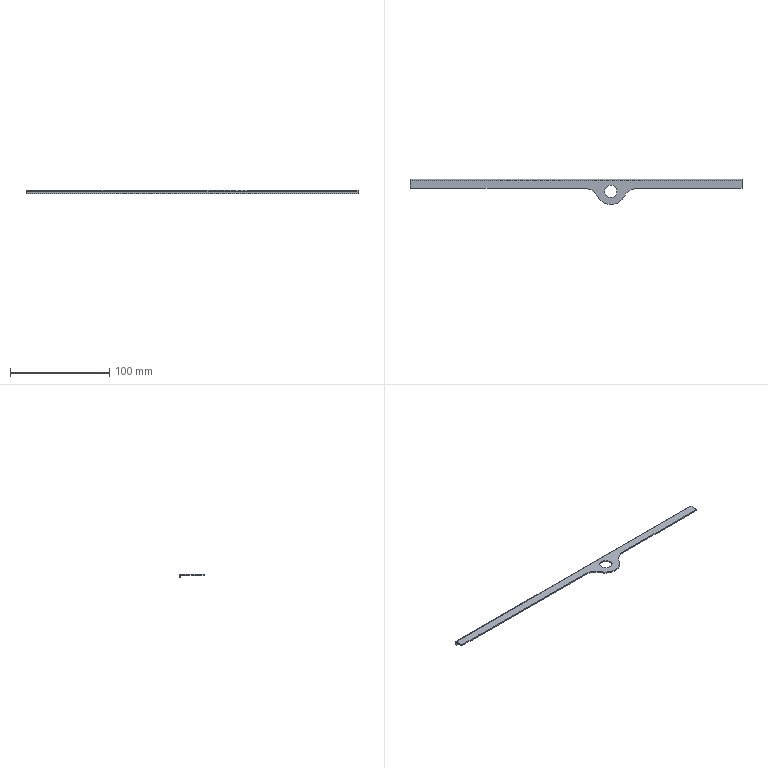Part | STEP file | gslz 2016.10.28-13_id1030_x_t | 1 solid | 17 faces | box 335 x 25.5 x 4 mm | volume 5252 mm3 | plane 10 | cylinder 7 | commonest cylinder face diameters 30 x3 4 x2 2 x1 12.3 x1
STEP:
#1=CARTESIAN_POINT('',(0.,0.,0.));
#2=DIRECTION('',(0.,0.,1.));
#3=DIRECTION('',(1.,0.,0.));
#4=AXIS2_PLACEMENT_3D('',#1,#2,#3);
#5=CARTESIAN_POINT('',(894.837,257.,0.));
#6=VERTEX_POINT('',#5);
#7=CARTESIAN_POINT('',(744.985,257.,0.));
#8=VERTEX_POINT('',#7);
#9=CARTESIAN_POINT('',(893.343,257.,0.));
#10=DIRECTION('',(-1.,0.,0.));
#11=VECTOR('',#10,1.);
#12=LINE('',#9,#11);
#13=CARTESIAN_POINT('',(893.343,257.,2.5));
#14=DIRECTION('',(0.,-1.,0.));
#15=DIRECTION('',(1.,0.,0.));
#16=AXIS2_PLACEMENT_3D('',#13,#14,#15);
#17=PLANE('',#16);
#18=CARTESIAN_POINT('',(0.,-2.5));
#19=DIRECTION('',(-1.,0.));
#20=VECTOR('',#19,1.);
#21=LINE('',#18,#20);
#22=(GEOMETRIC_REPRESENTATION_CONTEXT(2)PARAMETRIC_REPRESENTATION_CONTEXT()REPRESENTATION_CONTEXT('',''));
#23=DEFINITIONAL_REPRESENTATION('',(#21),#22);
#24=PCURVE('',#17,#23);
#25=CARTESIAN_POINT('',(3133.591,331.067,0.));
#26=DIRECTION('',(0.,0.,1.));
#27=DIRECTION('',(1.,0.,0.));
#28=AXIS2_PLACEMENT_3D('',#25,#26,#27);
#29=PLANE('',#28);
#30=CARTESIAN_POINT('',(-2240.248,-74.067));
#31=DIRECTION('',(-1.,0.));
#32=VECTOR('',#31,1.);
#33=LINE('',#30,#32);
#34=(GEOMETRIC_REPRESENTATION_CONTEXT(2)PARAMETRIC_REPRESENTATION_CONTEXT()REPRESENTATION_CONTEXT('',''));
#35=DEFINITIONAL_REPRESENTATION('',(#33),#34);
#36=PCURVE('',#29,#35);
#37=SURFACE_CURVE('',#12,(#24,#36),.PCURVE_S1.);
#38=EDGE_CURVE('',#6,#8,#37,.T.);
#39=ORIENTED_EDGE('',*,*,#38,.F.);
#40=CARTESIAN_POINT('',(894.837,257.,1.25));
#41=VERTEX_POINT('',#40);
#42=CARTESIAN_POINT('',(894.837,257.,2.5));
#43=DIRECTION('',(0.,0.,1.));
#44=VECTOR('',#43,1.);
#45=LINE('',#42,#44);
#46=CARTESIAN_POINT('',(1.493,0.));
#47=DIRECTION('',(0.,1.));
#48=VECTOR('',#47,1.);
#49=LINE('',#46,#48);
#50=(GEOMETRIC_REPRESENTATION_CONTEXT(2)PARAMETRIC_REPRESENTATION_CONTEXT()REPRESENTATION_CONTEXT('',''));
#51=DEFINITIONAL_REPRESENTATION('',(#49),#50);
#52=PCURVE('',#17,#51);
#53=CARTESIAN_POINT('',(894.837,242.,2.5));
#54=DIRECTION('',(0.,0.,-1.));
#55=DIRECTION('',(-1.,0.,0.));
#56=AXIS2_PLACEMENT_3D('',#53,#54,#55);
#57=CYLINDRICAL_SURFACE('',#56,15.);
#58=CARTESIAN_POINT('',(1.571,0.));
#59=DIRECTION('',(0.,-1.));
#60=VECTOR('',#59,1.);
#61=LINE('',#58,#60);
#62=(GEOMETRIC_REPRESENTATION_CONTEXT(2)PARAMETRIC_REPRESENTATION_CONTEXT()REPRESENTATION_CONTEXT('',''));
#63=DEFINITIONAL_REPRESENTATION('',(#61),#62);
#64=PCURVE('',#57,#63);
#65=SURFACE_CURVE('',#45,(#52,#64),.PCURVE_S1.);
#66=EDGE_CURVE('',#6,#41,#65,.T.);
#67=ORIENTED_EDGE('',*,*,#66,.T.);
#68=CARTESIAN_POINT('',(744.985,257.,1.25));
#69=VERTEX_POINT('',#68);
#70=CARTESIAN_POINT('',(3133.591,257.,1.25));
#71=DIRECTION('',(-1.,0.,0.));
#72=VECTOR('',#71,1.);
#73=LINE('',#70,#72);
#74=CARTESIAN_POINT('',(2240.248,-1.25));
#75=DIRECTION('',(-1.,0.));
#76=VECTOR('',#75,1.);
#77=LINE('',#74,#76);
#78=(GEOMETRIC_REPRESENTATION_CONTEXT(2)PARAMETRIC_REPRESENTATION_CONTEXT()REPRESENTATION_CONTEXT('',''));
#79=DEFINITIONAL_REPRESENTATION('',(#77),#78);
#80=PCURVE('',#17,#79);
#81=CARTESIAN_POINT('',(3133.591,331.067,1.25));
#82=DIRECTION('',(0.,0.,1.));
#83=DIRECTION('',(1.,0.,0.));
#84=AXIS2_PLACEMENT_3D('',#81,#82,#83);
#85=PLANE('',#84);
#86=CARTESIAN_POINT('',(0.,-74.067));
#87=DIRECTION('',(-1.,0.));
#88=VECTOR('',#87,1.);
#89=LINE('',#86,#88);
#90=(GEOMETRIC_REPRESENTATION_CONTEXT(2)PARAMETRIC_REPRESENTATION_CONTEXT()REPRESENTATION_CONTEXT('',''));
#91=DEFINITIONAL_REPRESENTATION('',(#89),#90);
#92=PCURVE('',#85,#91);
#93=SURFACE_CURVE('',#73,(#80,#92),.PCURVE_S1.);
#94=EDGE_CURVE('',#41,#69,#93,.T.);
#95=ORIENTED_EDGE('',*,*,#94,.T.);
#96=CARTESIAN_POINT('',(744.985,257.,2.5));
#97=DIRECTION('',(0.,0.,1.));
#98=VECTOR('',#97,1.);
#99=LINE('',#96,#98);
#100=CARTESIAN_POINT('',(-148.358,0.));
#101=DIRECTION('',(0.,1.));
#102=VECTOR('',#101,1.);
#103=LINE('',#100,#102);
#104=(GEOMETRIC_REPRESENTATION_CONTEXT(2)PARAMETRIC_REPRESENTATION_CONTEXT()REPRESENTATION_CONTEXT('',''));
#105=DEFINITIONAL_REPRESENTATION('',(#103),#104);
#106=PCURVE('',#17,#105);
#107=CARTESIAN_POINT('',(744.985,259.,2.5));
#108=DIRECTION('',(0.,0.,-1.));
#109=DIRECTION('',(-1.,0.,0.));
#110=AXIS2_PLACEMENT_3D('',#107,#108,#109);
#111=CYLINDRICAL_SURFACE('',#110,2.);
#112=CARTESIAN_POINT('',(4.712,0.));
#113=DIRECTION('',(0.,-1.));
#114=VECTOR('',#113,1.);
#115=LINE('',#112,#114);
#116=(GEOMETRIC_REPRESENTATION_CONTEXT(2)PARAMETRIC_REPRESENTATION_CONTEXT()REPRESENTATION_CONTEXT('',''));
#117=DEFINITIONAL_REPRESENTATION('',(#115),#116);
#118=PCURVE('',#111,#117);
#119=SURFACE_CURVE('',#99,(#106,#118),.PCURVE_S1.);
#120=EDGE_CURVE('',#8,#69,#119,.T.);
#121=ORIENTED_EDGE('',*,*,#120,.F.);
#122=EDGE_LOOP('',(#39,#67,#95,#121));
#123=FACE_BOUND('',#122,.T.);
#124=ADVANCED_FACE('',(#123),#17,.T.);
#125=CARTESIAN_POINT('',(718.925,265.,1.25));
#126=VERTEX_POINT('',#125);
#127=CARTESIAN_POINT('',(718.925,257.,1.25));
#128=VERTEX_POINT('',#127);
#129=CARTESIAN_POINT('',(718.925,331.067,1.25));
#130=DIRECTION('',(0.,-1.,0.));
#131=VECTOR('',#130,1.);
#132=LINE('',#129,#131);
#133=CARTESIAN_POINT('',(-2414.666,0.));
#134=DIRECTION('',(0.,-1.));
#135=VECTOR('',#134,1.);
#136=LINE('',#133,#135);
#137=(GEOMETRIC_REPRESENTATION_CONTEXT(2)PARAMETRIC_REPRESENTATION_CONTEXT()REPRESENTATION_CONTEXT('',''));
#138=DEFINITIONAL_REPRESENTATION('',(#136),#137);
#139=PCURVE('',#85,#138);
#140=CARTESIAN_POINT('',(718.925,261.5,-0.75));
#141=DIRECTION('',(1.,0.,0.));
#142=DIRECTION('',(0.,0.,-1.));
#143=AXIS2_PLACEMENT_3D('',#140,#141,#142);
#144=PLANE('',#143);
#145=CARTESIAN_POINT('',(-2.,69.567));
#146=DIRECTION('',(0.,-1.));
#147=VECTOR('',#146,1.);
#148=LINE('',#145,#147);
#149=(GEOMETRIC_REPRESENTATION_CONTEXT(2)PARAMETRIC_REPRESENTATION_CONTEXT()REPRESENTATION_CONTEXT('',''));
#150=DEFINITIONAL_REPRESENTATION('',(#148),#149);
#151=PCURVE('',#144,#150);
#152=SURFACE_CURVE('',#132,(#139,#151),.PCURVE_S1.);
#153=EDGE_CURVE('',#126,#128,#152,.T.);
#154=ORIENTED_EDGE('',*,*,#153,.T.);
#155=CARTESIAN_POINT('',(742.412,257.,1.25));
#156=VERTEX_POINT('',#155);
#157=CARTESIAN_POINT('',(3133.591,257.,1.25));
#158=DIRECTION('',(-1.,0.,0.));
#159=VECTOR('',#158,1.);
#160=LINE('',#157,#159);
#161=CARTESIAN_POINT('',(0.,-74.067));
#162=DIRECTION('',(-1.,0.));
#163=VECTOR('',#162,1.);
#164=LINE('',#161,#163);
#165=(GEOMETRIC_REPRESENTATION_CONTEXT(2)PARAMETRIC_REPRESENTATION_CONTEXT()REPRESENTATION_CONTEXT('',''));
#166=DEFINITIONAL_REPRESENTATION('',(#164),#165);
#167=PCURVE('',#85,#166);
#168=CARTESIAN_POINT('',(665.415,257.,2.5));
#169=DIRECTION('',(0.,1.,0.));
#170=DIRECTION('',(0.,0.,1.));
#171=AXIS2_PLACEMENT_3D('',#168,#169,#170);
#172=PLANE('',#171);
#173=CARTESIAN_POINT('',(-1.25,2468.176));
#174=DIRECTION('',(0.,-1.));
#175=VECTOR('',#174,1.);
#176=LINE('',#173,#175);
#177=(GEOMETRIC_REPRESENTATION_CONTEXT(2)PARAMETRIC_REPRESENTATION_CONTEXT()REPRESENTATION_CONTEXT('',''));
#178=DEFINITIONAL_REPRESENTATION('',(#176),#177);
#179=PCURVE('',#172,#178);
#180=SURFACE_CURVE('',#160,(#167,#179),.PCURVE_S1.);
#181=EDGE_CURVE('',#156,#128,#180,.T.);
#182=ORIENTED_EDGE('',*,*,#181,.F.);
#183=CARTESIAN_POINT('',(744.226,257.15,1.25));
#184=VERTEX_POINT('',#183);
#185=CARTESIAN_POINT('',(743.466,255.3,1.25));
#186=DIRECTION('',(0.,0.,1.));
#187=DIRECTION('',(1.,0.,0.));
#188=AXIS2_PLACEMENT_3D('',#185,#186,#187);
#189=CIRCLE('',#188,2.);
#190=CARTESIAN_POINT('',(-2390.126,-75.767));
#191=DIRECTION('',(1.,0.));
#192=AXIS2_PLACEMENT_2D('',#190,#191);
#193=CIRCLE('',#192,2.);
#194=(GEOMETRIC_REPRESENTATION_CONTEXT(2)PARAMETRIC_REPRESENTATION_CONTEXT()REPRESENTATION_CONTEXT('',''));
#195=DEFINITIONAL_REPRESENTATION('',(#193),#194);
#196=PCURVE('',#85,#195);
#197=CARTESIAN_POINT('',(743.466,255.3,2.5));
#198=DIRECTION('',(0.,0.,-1.));
#199=DIRECTION('',(-1.,0.,0.));
#200=AXIS2_PLACEMENT_3D('',#197,#198,#199);
#201=CYLINDRICAL_SURFACE('',#200,2.);
#202=CARTESIAN_POINT('',(3.142,1.25));
#203=DIRECTION('',(-1.,0.));
#204=VECTOR('',#203,1.);
#205=LINE('',#202,#204);
#206=(GEOMETRIC_REPRESENTATION_CONTEXT(2)PARAMETRIC_REPRESENTATION_CONTEXT()REPRESENTATION_CONTEXT('',''));
#207=DEFINITIONAL_REPRESENTATION('',(#205),#206);
#208=PCURVE('',#201,#207);
#209=SURFACE_CURVE('',#189,(#196,#208),.PCURVE_S1.);
#210=EDGE_CURVE('',#184,#156,#209,.T.);
#211=ORIENTED_EDGE('',*,*,#210,.F.);
#212=CARTESIAN_POINT('',(744.985,259.,1.25));
#213=DIRECTION('',(0.,0.,-1.));
#214=DIRECTION('',(1.,0.,0.));
#215=AXIS2_PLACEMENT_3D('',#212,#213,#214);
#216=CIRCLE('',#215,2.);
#217=CARTESIAN_POINT('',(-2386.606,-72.067));
#218=CARTESIAN_POINT('',(-2386.606,-75.531));
#219=CARTESIAN_POINT('',(-2389.606,-73.799));
#220=CARTESIAN_POINT('',(-2392.606,-72.067));
#221=CARTESIAN_POINT('',(-2389.606,-70.335));
#222=CARTESIAN_POINT('',(-2386.606,-68.603));
#223=CARTESIAN_POINT('',(-2386.606,-72.067));
#224=(BOUNDED_CURVE()B_SPLINE_CURVE(2,(#217,#218,#219,#220,#221,#222,#223),.UNSPECIFIED.,.T.,.F.)B_SPLINE_CURVE_WITH_KNOTS((1,2,2,2,2,1),(-2.094,0.,2.094,4.189,6.283,8.378),.UNSPECIFIED.)CURVE()GEOMETRIC_REPRESENTATION_ITEM()RATIONAL_B_SPLINE_CURVE((1.,0.5,1.,0.5,1.,0.5,1.))REPRESENTATION_ITEM(''));
#225=(GEOMETRIC_REPRESENTATION_CONTEXT(2)PARAMETRIC_REPRESENTATION_CONTEXT()REPRESENTATION_CONTEXT('',''));
#226=DEFINITIONAL_REPRESENTATION('',(#224),#225);
#227=PCURVE('',#85,#226);
#228=CARTESIAN_POINT('',(3.142,1.25));
#229=DIRECTION('',(1.,0.));
#230=VECTOR('',#229,1.);
#231=LINE('',#228,#230);
#232=(GEOMETRIC_REPRESENTATION_CONTEXT(2)PARAMETRIC_REPRESENTATION_CONTEXT()REPRESENTATION_CONTEXT('',''));
#233=DEFINITIONAL_REPRESENTATION('',(#231),#232);
#234=PCURVE('',#111,#233);
#235=SURFACE_CURVE('',#216,(#227,#234),.PCURVE_S1.);
#236=EDGE_CURVE('',#69,#184,#235,.T.);
#237=ORIENTED_EDGE('',*,*,#236,.F.);
#238=ORIENTED_EDGE('',*,*,#94,.F.);
#239=CARTESIAN_POINT('',(908.232,248.75,1.25));
#240=VERTEX_POINT('',#239);
#241=CARTESIAN_POINT('',(894.837,242.,1.25));
#242=DIRECTION('',(0.,0.,-1.));
#243=DIRECTION('',(1.,0.,0.));
#244=AXIS2_PLACEMENT_3D('',#241,#242,#243);
#245=CIRCLE('',#244,15.);
#246=CARTESIAN_POINT('',(-2223.754,-89.067));
#247=CARTESIAN_POINT('',(-2223.754,-115.047));
#248=CARTESIAN_POINT('',(-2246.254,-102.057));
#249=CARTESIAN_POINT('',(-2268.754,-89.067));
#250=CARTESIAN_POINT('',(-2246.254,-76.076));
#251=CARTESIAN_POINT('',(-2223.754,-63.086));
#252=CARTESIAN_POINT('',(-2223.754,-89.067));
#253=(BOUNDED_CURVE()B_SPLINE_CURVE(2,(#246,#247,#248,#249,#250,#251,#252),.UNSPECIFIED.,.T.,.F.)B_SPLINE_CURVE_WITH_KNOTS((1,2,2,2,2,1),(-2.094,0.,2.094,4.189,6.283,8.378),.UNSPECIFIED.)CURVE()GEOMETRIC_REPRESENTATION_ITEM()RATIONAL_B_SPLINE_CURVE((1.,0.5,1.,0.5,1.,0.5,1.))REPRESENTATION_ITEM(''));
#254=(GEOMETRIC_REPRESENTATION_CONTEXT(2)PARAMETRIC_REPRESENTATION_CONTEXT()REPRESENTATION_CONTEXT('',''));
#255=DEFINITIONAL_REPRESENTATION('',(#253),#254);
#256=PCURVE('',#85,#255);
#257=CARTESIAN_POINT('',(-3.142,1.25));
#258=DIRECTION('',(1.,0.));
#259=VECTOR('',#258,1.);
#260=LINE('',#257,#259);
#261=(GEOMETRIC_REPRESENTATION_CONTEXT(2)PARAMETRIC_REPRESENTATION_CONTEXT()REPRESENTATION_CONTEXT('',''));
#262=DEFINITIONAL_REPRESENTATION('',(#260),#261);
#263=PCURVE('',#57,#262);
#264=SURFACE_CURVE('',#245,(#256,#263),.PCURVE_S1.);
#265=EDGE_CURVE('',#41,#240,#264,.T.);
#266=ORIENTED_EDGE('',*,*,#265,.T.);
#267=CARTESIAN_POINT('',(935.023,248.75,1.25));
#268=VERTEX_POINT('',#267);
#269=CARTESIAN_POINT('',(921.628,255.5,1.25));
#270=DIRECTION('',(0.,0.,1.));
#271=DIRECTION('',(1.,0.,0.));
#272=AXIS2_PLACEMENT_3D('',#269,#270,#271);
#273=CIRCLE('',#272,15.);
#274=CARTESIAN_POINT('',(-2211.964,-75.567));
#275=DIRECTION('',(1.,0.));
#276=AXIS2_PLACEMENT_2D('',#274,#275);
#277=CIRCLE('',#276,15.);
#278=(GEOMETRIC_REPRESENTATION_CONTEXT(2)PARAMETRIC_REPRESENTATION_CONTEXT()REPRESENTATION_CONTEXT('',''));
#279=DEFINITIONAL_REPRESENTATION('',(#277),#278);
#280=PCURVE('',#85,#279);
#281=CARTESIAN_POINT('',(921.628,255.5,2.5));
#282=DIRECTION('',(0.,0.,-1.));
#283=DIRECTION('',(-1.,0.,0.));
#284=AXIS2_PLACEMENT_3D('',#281,#282,#283);
#285=CYLINDRICAL_SURFACE('',#284,15.);
#286=CARTESIAN_POINT('',(9.425,1.25));
#287=DIRECTION('',(-1.,0.));
#288=VECTOR('',#287,1.);
#289=LINE('',#286,#288);
#290=(GEOMETRIC_REPRESENTATION_CONTEXT(2)PARAMETRIC_REPRESENTATION_CONTEXT()REPRESENTATION_CONTEXT('',''));
#291=DEFINITIONAL_REPRESENTATION('',(#289),#290);
#292=PCURVE('',#285,#291);
#293=SURFACE_CURVE('',#273,(#280,#292),.PCURVE_S1.);
#294=EDGE_CURVE('',#240,#268,#293,.T.);
#295=ORIENTED_EDGE('',*,*,#294,.T.);
#296=CARTESIAN_POINT('',(948.418,257.,1.25));
#297=VERTEX_POINT('',#296);
#298=CARTESIAN_POINT('',(948.418,242.,1.25));
#299=DIRECTION('',(0.,0.,-1.));
#300=DIRECTION('',(1.,0.,0.));
#301=AXIS2_PLACEMENT_3D('',#298,#299,#300);
#302=CIRCLE('',#301,15.);
#303=CARTESIAN_POINT('',(-2170.173,-89.067));
#304=CARTESIAN_POINT('',(-2170.173,-115.047));
#305=CARTESIAN_POINT('',(-2192.673,-102.057));
#306=CARTESIAN_POINT('',(-2215.173,-89.067));
#307=CARTESIAN_POINT('',(-2192.673,-76.076));
#308=CARTESIAN_POINT('',(-2170.173,-63.086));
#309=CARTESIAN_POINT('',(-2170.173,-89.067));
#310=(BOUNDED_CURVE()B_SPLINE_CURVE(2,(#303,#304,#305,#306,#307,#308,#309),.UNSPECIFIED.,.T.,.F.)B_SPLINE_CURVE_WITH_KNOTS((1,2,2,2,2,1),(-2.094,0.,2.094,4.189,6.283,8.378),.UNSPECIFIED.)CURVE()GEOMETRIC_REPRESENTATION_ITEM()RATIONAL_B_SPLINE_CURVE((1.,0.5,1.,0.5,1.,0.5,1.))REPRESENTATION_ITEM(''));
#311=(GEOMETRIC_REPRESENTATION_CONTEXT(2)PARAMETRIC_REPRESENTATION_CONTEXT()REPRESENTATION_CONTEXT('',''));
#312=DEFINITIONAL_REPRESENTATION('',(#310),#311);
#313=PCURVE('',#85,#312);
#314=CARTESIAN_POINT('',(948.418,242.,2.5));
#315=DIRECTION('',(0.,0.,-1.));
#316=DIRECTION('',(-1.,0.,0.));
#317=AXIS2_PLACEMENT_3D('',#314,#315,#316);
#318=CYLINDRICAL_SURFACE('',#317,15.);
#319=CARTESIAN_POINT('',(-3.142,1.25));
#320=DIRECTION('',(1.,0.));
#321=VECTOR('',#320,1.);
#322=LINE('',#319,#321);
#323=(GEOMETRIC_REPRESENTATION_CONTEXT(2)PARAMETRIC_REPRESENTATION_CONTEXT()REPRESENTATION_CONTEXT('',''));
#324=DEFINITIONAL_REPRESENTATION('',(#322),#323);
#325=PCURVE('',#318,#324);
#326=SURFACE_CURVE('',#302,(#313,#325),.PCURVE_S1.);
#327=EDGE_CURVE('',#268,#297,#326,.T.);
#328=ORIENTED_EDGE('',*,*,#327,.T.);
#329=CARTESIAN_POINT('',(1053.925,257.,1.25));
#330=VERTEX_POINT('',#329);
#331=CARTESIAN_POINT('',(3133.591,257.,1.25));
#332=DIRECTION('',(-1.,0.,0.));
#333=VECTOR('',#332,1.);
#334=LINE('',#331,#333);
#335=CARTESIAN_POINT('',(0.,-74.067));
#336=DIRECTION('',(-1.,0.));
#337=VECTOR('',#336,1.);
#338=LINE('',#335,#337);
#339=(GEOMETRIC_REPRESENTATION_CONTEXT(2)PARAMETRIC_REPRESENTATION_CONTEXT()REPRESENTATION_CONTEXT('',''));
#340=DEFINITIONAL_REPRESENTATION('',(#338),#339);
#341=PCURVE('',#85,#340);
#342=CARTESIAN_POINT('',(928.783,257.,0.));
#343=DIRECTION('',(0.,-1.,0.));
#344=DIRECTION('',(0.,0.,-1.));
#345=AXIS2_PLACEMENT_3D('',#342,#343,#344);
#346=PLANE('',#345);
#347=CARTESIAN_POINT('',(-1.25,2204.808));
#348=DIRECTION('',(0.,-1.));
#349=VECTOR('',#348,1.);
#350=LINE('',#347,#349);
#351=(GEOMETRIC_REPRESENTATION_CONTEXT(2)PARAMETRIC_REPRESENTATION_CONTEXT()REPRESENTATION_CONTEXT('',''));
#352=DEFINITIONAL_REPRESENTATION('',(#350),#351);
#353=PCURVE('',#346,#352);
#354=SURFACE_CURVE('',#334,(#341,#353),.PCURVE_S1.);
#355=EDGE_CURVE('',#330,#297,#354,.T.);
#356=ORIENTED_EDGE('',*,*,#355,.F.);
#357=CARTESIAN_POINT('',(1053.925,265.,1.25));
#358=VERTEX_POINT('',#357);
#359=CARTESIAN_POINT('',(1053.925,263.5,1.25));
#360=DIRECTION('',(0.,-1.,0.));
#361=VECTOR('',#360,1.);
#362=LINE('',#359,#361);
#363=CARTESIAN_POINT('',(-2079.666,-67.567));
#364=DIRECTION('',(0.,-1.));
#365=VECTOR('',#364,1.);
#366=LINE('',#363,#365);
#367=(GEOMETRIC_REPRESENTATION_CONTEXT(2)PARAMETRIC_REPRESENTATION_CONTEXT()REPRESENTATION_CONTEXT('',''));
#368=DEFINITIONAL_REPRESENTATION('',(#366),#367);
#369=PCURVE('',#85,#368);
#370=CARTESIAN_POINT('',(1053.925,263.5,0.625));
#371=DIRECTION('',(-1.,0.,0.));
#372=DIRECTION('',(0.,0.,1.));
#373=AXIS2_PLACEMENT_3D('',#370,#371,#372);
#374=PLANE('',#373);
#375=CARTESIAN_POINT('',(0.625,0.));
#376=DIRECTION('',(0.,-1.));
#377=VECTOR('',#376,1.);
#378=LINE('',#375,#377);
#379=(GEOMETRIC_REPRESENTATION_CONTEXT(2)PARAMETRIC_REPRESENTATION_CONTEXT()REPRESENTATION_CONTEXT('',''));
#380=DEFINITIONAL_REPRESENTATION('',(#378),#379);
#381=PCURVE('',#374,#380);
#382=SURFACE_CURVE('',#362,(#369,#381),.PCURVE_S1.);
#383=EDGE_CURVE('',#358,#330,#382,.T.);
#384=ORIENTED_EDGE('',*,*,#383,.F.);
#385=CARTESIAN_POINT('',(713.824,265.,1.25));
#386=DIRECTION('',(-1.,0.,0.));
#387=VECTOR('',#386,1.);
#388=LINE('',#385,#387);
#389=CARTESIAN_POINT('',(-2419.767,-66.067));
#390=DIRECTION('',(-1.,0.));
#391=VECTOR('',#390,1.);
#392=LINE('',#389,#391);
#393=(GEOMETRIC_REPRESENTATION_CONTEXT(2)PARAMETRIC_REPRESENTATION_CONTEXT()REPRESENTATION_CONTEXT('',''));
#394=DEFINITIONAL_REPRESENTATION('',(#392),#393);
#395=PCURVE('',#85,#394);
#396=CARTESIAN_POINT('',(3133.591,265.,0.25));
#397=DIRECTION('',(-1.,0.,0.));
#398=DIRECTION('',(0.,-1.,0.));
#399=AXIS2_PLACEMENT_3D('',#396,#397,#398);
#400=CYLINDRICAL_SURFACE('',#399,1.);
#401=CARTESIAN_POINT('',(1.571,2419.767));
#402=DIRECTION('',(0.,1.));
#403=VECTOR('',#402,1.);
#404=LINE('',#401,#403);
#405=(GEOMETRIC_REPRESENTATION_CONTEXT(2)PARAMETRIC_REPRESENTATION_CONTEXT()REPRESENTATION_CONTEXT('',''));
#406=DEFINITIONAL_REPRESENTATION('',(#404),#405);
#407=PCURVE('',#400,#406);
#408=SURFACE_CURVE('',#388,(#395,#407),.PCURVE_S1.);
#409=EDGE_CURVE('',#358,#126,#408,.T.);
#410=ORIENTED_EDGE('',*,*,#409,.T.);
#411=EDGE_LOOP('',(#154,#182,#211,#237,#238,#266,#295,#328,#356,#384,#410));
#412=FACE_BOUND('',#411,.T.);
#413=CARTESIAN_POINT('',(927.778,254.,1.25));
#414=VERTEX_POINT('',#413);
#415=CARTESIAN_POINT('',(921.628,254.,1.25));
#416=DIRECTION('',(0.,0.,1.));
#417=DIRECTION('',(1.,0.,0.));
#418=AXIS2_PLACEMENT_3D('',#415,#416,#417);
#419=CIRCLE('',#418,6.15);
#420=CARTESIAN_POINT('',(-2211.964,-77.067));
#421=DIRECTION('',(1.,0.));
#422=AXIS2_PLACEMENT_2D('',#420,#421);
#423=CIRCLE('',#422,6.15);
#424=(GEOMETRIC_REPRESENTATION_CONTEXT(2)PARAMETRIC_REPRESENTATION_CONTEXT()REPRESENTATION_CONTEXT('',''));
#425=DEFINITIONAL_REPRESENTATION('',(#423),#424);
#426=PCURVE('',#85,#425);
#427=CARTESIAN_POINT('',(921.628,254.,2.5));
#428=DIRECTION('',(0.,0.,-1.));
#429=DIRECTION('',(-1.,0.,0.));
#430=AXIS2_PLACEMENT_3D('',#427,#428,#429);
#431=CYLINDRICAL_SURFACE('',#430,6.15);
#432=CARTESIAN_POINT('',(9.425,1.25));
#433=DIRECTION('',(-1.,0.));
#434=VECTOR('',#433,1.);
#435=LINE('',#432,#434);
#436=(GEOMETRIC_REPRESENTATION_CONTEXT(2)PARAMETRIC_REPRESENTATION_CONTEXT()REPRESENTATION_CONTEXT('',''));
#437=DEFINITIONAL_REPRESENTATION('',(#435),#436);
#438=PCURVE('',#431,#437);
#439=SURFACE_CURVE('',#419,(#426,#438),.PCURVE_S1.);
#440=EDGE_CURVE('',#414,#414,#439,.T.);
#441=ORIENTED_EDGE('',*,*,#440,.F.);
#442=EDGE_LOOP('',(#441));
#443=FACE_BOUND('',#442,.T.);
#444=ADVANCED_FACE('',(#412,#443),#85,.T.);
#445=CARTESIAN_POINT('',(742.412,257.,0.));
#446=VERTEX_POINT('',#445);
#447=CARTESIAN_POINT('',(718.925,257.,0.));
#448=VERTEX_POINT('',#447);
#449=CARTESIAN_POINT('',(654.415,257.,0.));
#450=DIRECTION('',(-1.,0.,0.));
#451=VECTOR('',#450,1.);
#452=LINE('',#449,#451);
#453=CARTESIAN_POINT('',(-2479.176,-74.067));
#454=DIRECTION('',(-1.,0.));
#455=VECTOR('',#454,1.);
#456=LINE('',#453,#455);
#457=(GEOMETRIC_REPRESENTATION_CONTEXT(2)PARAMETRIC_REPRESENTATION_CONTEXT()REPRESENTATION_CONTEXT('',''));
#458=DEFINITIONAL_REPRESENTATION('',(#456),#457);
#459=PCURVE('',#29,#458);
#460=CARTESIAN_POINT('',(-2.5,-11.));
#461=DIRECTION('',(0.,-1.));
#462=VECTOR('',#461,1.);
#463=LINE('',#460,#462);
#464=(GEOMETRIC_REPRESENTATION_CONTEXT(2)PARAMETRIC_REPRESENTATION_CONTEXT()REPRESENTATION_CONTEXT('',''));
#465=DEFINITIONAL_REPRESENTATION('',(#463),#464);
#466=PCURVE('',#172,#465);
#467=SURFACE_CURVE('',#452,(#459,#466),.PCURVE_S1.);
#468=EDGE_CURVE('',#446,#448,#467,.T.);
#469=ORIENTED_EDGE('',*,*,#468,.T.);
#470=CARTESIAN_POINT('',(718.925,264.75,0.));
#471=VERTEX_POINT('',#470);
#472=CARTESIAN_POINT('',(718.925,331.067,0.));
#473=DIRECTION('',(0.,-1.,0.));
#474=VECTOR('',#473,1.);
#475=LINE('',#472,#474);
#476=CARTESIAN_POINT('',(-2414.666,0.));
#477=DIRECTION('',(0.,-1.));
#478=VECTOR('',#477,1.);
#479=LINE('',#476,#478);
#480=(GEOMETRIC_REPRESENTATION_CONTEXT(2)PARAMETRIC_REPRESENTATION_CONTEXT()REPRESENTATION_CONTEXT('',''));
#481=DEFINITIONAL_REPRESENTATION('',(#479),#480);
#482=PCURVE('',#29,#481);
#483=CARTESIAN_POINT('',(-0.75,69.567));
#484=DIRECTION('',(0.,-1.));
#485=VECTOR('',#484,1.);
#486=LINE('',#483,#485);
#487=(GEOMETRIC_REPRESENTATION_CONTEXT(2)PARAMETRIC_REPRESENTATION_CONTEXT()REPRESENTATION_CONTEXT('',''));
#488=DEFINITIONAL_REPRESENTATION('',(#486),#487);
#489=PCURVE('',#144,#488);
#490=SURFACE_CURVE('',#475,(#482,#489),.PCURVE_S1.);
#491=EDGE_CURVE('',#471,#448,#490,.T.);
#492=ORIENTED_EDGE('',*,*,#491,.F.);
#493=CARTESIAN_POINT('',(1053.925,264.75,0.));
#494=VERTEX_POINT('',#493);
#495=CARTESIAN_POINT('',(2893.925,264.75,0.));
#496=DIRECTION('',(-1.,0.,0.));
#497=VECTOR('',#496,1.);
#498=LINE('',#495,#497);
#499=CARTESIAN_POINT('',(-239.666,-66.317));
#500=DIRECTION('',(-1.,0.));
#501=VECTOR('',#500,1.);
#502=LINE('',#499,#501);
#503=(GEOMETRIC_REPRESENTATION_CONTEXT(2)PARAMETRIC_REPRESENTATION_CONTEXT()REPRESENTATION_CONTEXT('',''));
#504=DEFINITIONAL_REPRESENTATION('',(#502),#503);
#505=PCURVE('',#29,#504);
#506=CARTESIAN_POINT('',(2893.925,264.75,-135.834));
#507=DIRECTION('',(0.,1.,0.));
#508=DIRECTION('',(1.,0.,0.));
#509=AXIS2_PLACEMENT_3D('',#506,#507,#508);
#510=PLANE('',#509);
#511=CARTESIAN_POINT('',(0.,-135.834));
#512=DIRECTION('',(-1.,0.));
#513=VECTOR('',#512,1.);
#514=LINE('',#511,#513);
#515=(GEOMETRIC_REPRESENTATION_CONTEXT(2)PARAMETRIC_REPRESENTATION_CONTEXT()REPRESENTATION_CONTEXT('',''));
#516=DEFINITIONAL_REPRESENTATION('',(#514),#515);
#517=PCURVE('',#510,#516);
#518=SURFACE_CURVE('',#498,(#505,#517),.PCURVE_S1.);
#519=EDGE_CURVE('',#494,#471,#518,.T.);
#520=ORIENTED_EDGE('',*,*,#519,.F.);
#521=CARTESIAN_POINT('',(1053.925,257.,0.));
#522=VERTEX_POINT('',#521);
#523=CARTESIAN_POINT('',(1053.925,263.5,0.));
#524=DIRECTION('',(0.,1.,0.));
#525=VECTOR('',#524,1.);
#526=LINE('',#523,#525);
#527=CARTESIAN_POINT('',(-2079.666,-67.567));
#528=DIRECTION('',(0.,1.));
#529=VECTOR('',#528,1.);
#530=LINE('',#527,#529);
#531=(GEOMETRIC_REPRESENTATION_CONTEXT(2)PARAMETRIC_REPRESENTATION_CONTEXT()REPRESENTATION_CONTEXT('',''));
#532=DEFINITIONAL_REPRESENTATION('',(#530),#531);
#533=PCURVE('',#29,#532);
#534=CARTESIAN_POINT('',(-0.625,0.));
#535=DIRECTION('',(0.,1.));
#536=VECTOR('',#535,1.);
#537=LINE('',#534,#536);
#538=(GEOMETRIC_REPRESENTATION_CONTEXT(2)PARAMETRIC_REPRESENTATION_CONTEXT()REPRESENTATION_CONTEXT('',''));
#539=DEFINITIONAL_REPRESENTATION('',(#537),#538);
#540=PCURVE('',#374,#539);
#541=SURFACE_CURVE('',#526,(#533,#540),.PCURVE_S1.);
#542=EDGE_CURVE('',#522,#494,#541,.T.);
#543=ORIENTED_EDGE('',*,*,#542,.F.);
#544=CARTESIAN_POINT('',(948.418,257.,0.));
#545=VERTEX_POINT('',#544);
#546=CARTESIAN_POINT('',(928.783,257.,0.));
#547=DIRECTION('',(-1.,0.,0.));
#548=VECTOR('',#547,1.);
#549=LINE('',#546,#548);
#550=CARTESIAN_POINT('',(-2204.808,-74.067));
#551=DIRECTION('',(-1.,0.));
#552=VECTOR('',#551,1.);
#553=LINE('',#550,#552);
#554=(GEOMETRIC_REPRESENTATION_CONTEXT(2)PARAMETRIC_REPRESENTATION_CONTEXT()REPRESENTATION_CONTEXT('',''));
#555=DEFINITIONAL_REPRESENTATION('',(#553),#554);
#556=PCURVE('',#29,#555);
#557=CARTESIAN_POINT('',(0.,0.));
#558=DIRECTION('',(0.,-1.));
#559=VECTOR('',#558,1.);
#560=LINE('',#557,#559);
#561=(GEOMETRIC_REPRESENTATION_CONTEXT(2)PARAMETRIC_REPRESENTATION_CONTEXT()REPRESENTATION_CONTEXT('',''));
#562=DEFINITIONAL_REPRESENTATION('',(#560),#561);
#563=PCURVE('',#346,#562);
#564=SURFACE_CURVE('',#549,(#556,#563),.PCURVE_S1.);
#565=EDGE_CURVE('',#522,#545,#564,.T.);
#566=ORIENTED_EDGE('',*,*,#565,.T.);
#567=CARTESIAN_POINT('',(935.023,248.75,0.));
#568=VERTEX_POINT('',#567);
#569=CARTESIAN_POINT('',(948.418,242.,0.));
#570=DIRECTION('',(0.,0.,1.));
#571=DIRECTION('',(1.,0.,0.));
#572=AXIS2_PLACEMENT_3D('',#569,#570,#571);
#573=CIRCLE('',#572,15.);
#574=CARTESIAN_POINT('',(-2185.173,-89.067));
#575=DIRECTION('',(1.,0.));
#576=AXIS2_PLACEMENT_2D('',#574,#575);
#577=CIRCLE('',#576,15.);
#578=(GEOMETRIC_REPRESENTATION_CONTEXT(2)PARAMETRIC_REPRESENTATION_CONTEXT()REPRESENTATION_CONTEXT('',''));
#579=DEFINITIONAL_REPRESENTATION('',(#577),#578);
#580=PCURVE('',#29,#579);
#581=CARTESIAN_POINT('',(3.142,2.5));
#582=DIRECTION('',(-1.,0.));
#583=VECTOR('',#582,1.);
#584=LINE('',#581,#583);
#585=(GEOMETRIC_REPRESENTATION_CONTEXT(2)PARAMETRIC_REPRESENTATION_CONTEXT()REPRESENTATION_CONTEXT('',''));
#586=DEFINITIONAL_REPRESENTATION('',(#584),#585);
#587=PCURVE('',#318,#586);
#588=SURFACE_CURVE('',#573,(#580,#587),.PCURVE_S1.);
#589=EDGE_CURVE('',#545,#568,#588,.T.);
#590=ORIENTED_EDGE('',*,*,#589,.T.);
#591=CARTESIAN_POINT('',(908.232,248.75,0.));
#592=VERTEX_POINT('',#591);
#593=CARTESIAN_POINT('',(921.628,255.5,0.));
#594=DIRECTION('',(0.,0.,-1.));
#595=DIRECTION('',(1.,0.,0.));
#596=AXIS2_PLACEMENT_3D('',#593,#594,#595);
#597=CIRCLE('',#596,15.);
#598=CARTESIAN_POINT('',(-2196.964,-75.567));
#599=CARTESIAN_POINT('',(-2196.964,-101.547));
#600=CARTESIAN_POINT('',(-2219.464,-88.557));
#601=CARTESIAN_POINT('',(-2241.964,-75.567));
#602=CARTESIAN_POINT('',(-2219.464,-62.576));
#603=CARTESIAN_POINT('',(-2196.964,-49.586));
#604=CARTESIAN_POINT('',(-2196.964,-75.567));
#605=(BOUNDED_CURVE()B_SPLINE_CURVE(2,(#598,#599,#600,#601,#602,#603,#604),.UNSPECIFIED.,.T.,.F.)B_SPLINE_CURVE_WITH_KNOTS((1,2,2,2,2,1),(-2.094,0.,2.094,4.189,6.283,8.378),.UNSPECIFIED.)CURVE()GEOMETRIC_REPRESENTATION_ITEM()RATIONAL_B_SPLINE_CURVE((1.,0.5,1.,0.5,1.,0.5,1.))REPRESENTATION_ITEM(''));
#606=(GEOMETRIC_REPRESENTATION_CONTEXT(2)PARAMETRIC_REPRESENTATION_CONTEXT()REPRESENTATION_CONTEXT('',''));
#607=DEFINITIONAL_REPRESENTATION('',(#605),#606);
#608=PCURVE('',#29,#607);
#609=CARTESIAN_POINT('',(3.142,2.5));
#610=DIRECTION('',(1.,0.));
#611=VECTOR('',#610,1.);
#612=LINE('',#609,#611);
#613=(GEOMETRIC_REPRESENTATION_CONTEXT(2)PARAMETRIC_REPRESENTATION_CONTEXT()REPRESENTATION_CONTEXT('',''));
#614=DEFINITIONAL_REPRESENTATION('',(#612),#613);
#615=PCURVE('',#285,#614);
#616=SURFACE_CURVE('',#597,(#608,#615),.PCURVE_S1.);
#617=EDGE_CURVE('',#568,#592,#616,.T.);
#618=ORIENTED_EDGE('',*,*,#617,.T.);
#619=CARTESIAN_POINT('',(894.837,242.,0.));
#620=DIRECTION('',(0.,0.,1.));
#621=DIRECTION('',(1.,0.,0.));
#622=AXIS2_PLACEMENT_3D('',#619,#620,#621);
#623=CIRCLE('',#622,15.);
#624=CARTESIAN_POINT('',(-2238.754,-89.067));
#625=DIRECTION('',(1.,0.));
#626=AXIS2_PLACEMENT_2D('',#624,#625);
#627=CIRCLE('',#626,15.);
#628=(GEOMETRIC_REPRESENTATION_CONTEXT(2)PARAMETRIC_REPRESENTATION_CONTEXT()REPRESENTATION_CONTEXT('',''));
#629=DEFINITIONAL_REPRESENTATION('',(#627),#628);
#630=PCURVE('',#29,#629);
#631=CARTESIAN_POINT('',(3.142,2.5));
#632=DIRECTION('',(-1.,0.));
#633=VECTOR('',#632,1.);
#634=LINE('',#631,#633);
#635=(GEOMETRIC_REPRESENTATION_CONTEXT(2)PARAMETRIC_REPRESENTATION_CONTEXT()REPRESENTATION_CONTEXT('',''));
#636=DEFINITIONAL_REPRESENTATION('',(#634),#635);
#637=PCURVE('',#57,#636);
#638=SURFACE_CURVE('',#623,(#630,#637),.PCURVE_S1.);
#639=EDGE_CURVE('',#592,#6,#638,.T.);
#640=ORIENTED_EDGE('',*,*,#639,.T.);
#641=ORIENTED_EDGE('',*,*,#38,.T.);
#642=CARTESIAN_POINT('',(744.226,257.15,0.));
#643=VERTEX_POINT('',#642);
#644=CARTESIAN_POINT('',(744.985,259.,0.));
#645=DIRECTION('',(0.,0.,1.));
#646=DIRECTION('',(1.,0.,0.));
#647=AXIS2_PLACEMENT_3D('',#644,#645,#646);
#648=CIRCLE('',#647,2.);
#649=CARTESIAN_POINT('',(-2388.606,-72.067));
#650=DIRECTION('',(1.,0.));
#651=AXIS2_PLACEMENT_2D('',#649,#650);
#652=CIRCLE('',#651,2.);
#653=(GEOMETRIC_REPRESENTATION_CONTEXT(2)PARAMETRIC_REPRESENTATION_CONTEXT()REPRESENTATION_CONTEXT('',''));
#654=DEFINITIONAL_REPRESENTATION('',(#652),#653);
#655=PCURVE('',#29,#654);
#656=CARTESIAN_POINT('',(9.425,2.5));
#657=DIRECTION('',(-1.,0.));
#658=VECTOR('',#657,1.);
#659=LINE('',#656,#658);
#660=(GEOMETRIC_REPRESENTATION_CONTEXT(2)PARAMETRIC_REPRESENTATION_CONTEXT()REPRESENTATION_CONTEXT('',''));
#661=DEFINITIONAL_REPRESENTATION('',(#659),#660);
#662=PCURVE('',#111,#661);
#663=SURFACE_CURVE('',#648,(#655,#662),.PCURVE_S1.);
#664=EDGE_CURVE('',#643,#8,#663,.T.);
#665=ORIENTED_EDGE('',*,*,#664,.F.);
#666=CARTESIAN_POINT('',(743.466,255.3,0.));
#667=DIRECTION('',(0.,0.,-1.));
#668=DIRECTION('',(1.,0.,0.));
#669=AXIS2_PLACEMENT_3D('',#666,#667,#668);
#670=CIRCLE('',#669,2.);
#671=CARTESIAN_POINT('',(-2388.126,-75.767));
#672=CARTESIAN_POINT('',(-2388.126,-79.231));
#673=CARTESIAN_POINT('',(-2391.126,-77.499));
#674=CARTESIAN_POINT('',(-2394.126,-75.767));
#675=CARTESIAN_POINT('',(-2391.126,-74.035));
#676=CARTESIAN_POINT('',(-2388.126,-72.303));
#677=CARTESIAN_POINT('',(-2388.126,-75.767));
#678=(BOUNDED_CURVE()B_SPLINE_CURVE(2,(#671,#672,#673,#674,#675,#676,#677),.UNSPECIFIED.,.T.,.F.)B_SPLINE_CURVE_WITH_KNOTS((1,2,2,2,2,1),(-2.094,0.,2.094,4.189,6.283,8.378),.UNSPECIFIED.)CURVE()GEOMETRIC_REPRESENTATION_ITEM()RATIONAL_B_SPLINE_CURVE((1.,0.5,1.,0.5,1.,0.5,1.))REPRESENTATION_ITEM(''));
#679=(GEOMETRIC_REPRESENTATION_CONTEXT(2)PARAMETRIC_REPRESENTATION_CONTEXT()REPRESENTATION_CONTEXT('',''));
#680=DEFINITIONAL_REPRESENTATION('',(#678),#679);
#681=PCURVE('',#29,#680);
#682=CARTESIAN_POINT('',(-3.142,2.5));
#683=DIRECTION('',(1.,0.));
#684=VECTOR('',#683,1.);
#685=LINE('',#682,#684);
#686=(GEOMETRIC_REPRESENTATION_CONTEXT(2)PARAMETRIC_REPRESENTATION_CONTEXT()REPRESENTATION_CONTEXT('',''));
#687=DEFINITIONAL_REPRESENTATION('',(#685),#686);
#688=PCURVE('',#201,#687);
#689=SURFACE_CURVE('',#670,(#681,#688),.PCURVE_S1.);
#690=EDGE_CURVE('',#446,#643,#689,.T.);
#691=ORIENTED_EDGE('',*,*,#690,.F.);
#692=EDGE_LOOP('',(#469,#492,#520,#543,#566,#590,#618,#640,#641,#665,#691));
#693=FACE_BOUND('',#692,.T.);
#694=CARTESIAN_POINT('',(927.778,254.,0.));
#695=VERTEX_POINT('',#694);
#696=CARTESIAN_POINT('',(921.628,254.,0.));
#697=DIRECTION('',(0.,0.,-1.));
#698=DIRECTION('',(1.,0.,0.));
#699=AXIS2_PLACEMENT_3D('',#696,#697,#698);
#700=CIRCLE('',#699,6.15);
#701=CARTESIAN_POINT('',(-2205.814,-77.067));
#702=CARTESIAN_POINT('',(-2205.814,-87.719));
#703=CARTESIAN_POINT('',(-2215.039,-82.393));
#704=CARTESIAN_POINT('',(-2224.264,-77.067));
#705=CARTESIAN_POINT('',(-2215.039,-71.741));
#706=CARTESIAN_POINT('',(-2205.814,-66.415));
#707=CARTESIAN_POINT('',(-2205.814,-77.067));
#708=(BOUNDED_CURVE()B_SPLINE_CURVE(2,(#701,#702,#703,#704,#705,#706,#707),.UNSPECIFIED.,.T.,.F.)B_SPLINE_CURVE_WITH_KNOTS((1,2,2,2,2,1),(-2.094,0.,2.094,4.189,6.283,8.378),.UNSPECIFIED.)CURVE()GEOMETRIC_REPRESENTATION_ITEM()RATIONAL_B_SPLINE_CURVE((1.,0.5,1.,0.5,1.,0.5,1.))REPRESENTATION_ITEM(''));
#709=(GEOMETRIC_REPRESENTATION_CONTEXT(2)PARAMETRIC_REPRESENTATION_CONTEXT()REPRESENTATION_CONTEXT('',''));
#710=DEFINITIONAL_REPRESENTATION('',(#708),#709);
#711=PCURVE('',#29,#710);
#712=CARTESIAN_POINT('',(3.142,2.5));
#713=DIRECTION('',(1.,0.));
#714=VECTOR('',#713,1.);
#715=LINE('',#712,#714);
#716=(GEOMETRIC_REPRESENTATION_CONTEXT(2)PARAMETRIC_REPRESENTATION_CONTEXT()REPRESENTATION_CONTEXT('',''));
#717=DEFINITIONAL_REPRESENTATION('',(#715),#716);
#718=PCURVE('',#431,#717);
#719=SURFACE_CURVE('',#700,(#711,#718),.PCURVE_S1.);
#720=EDGE_CURVE('',#695,#695,#719,.T.);
#721=ORIENTED_EDGE('',*,*,#720,.F.);
#722=EDGE_LOOP('',(#721));
#723=FACE_BOUND('',#722,.T.);
#724=ADVANCED_FACE('',(#693,#723),#29,.F.);
#725=ORIENTED_EDGE('',*,*,#440,.F.);
#726=CARTESIAN_POINT('',(927.778,254.,1.25));
#727=CARTESIAN_POINT('',(927.778,254.,0.));
#728=B_SPLINE_CURVE_WITH_KNOTS('',1,(#726,#727),.UNSPECIFIED.,.F.,.F.,(2,2),(1.25,2.5),.PIECEWISE_BEZIER_KNOTS.);
#729=CARTESIAN_POINT('',(9.425,0.));
#730=DIRECTION('',(0.,1.));
#731=VECTOR('',#730,1.);
#732=LINE('',#729,#731);
#733=(GEOMETRIC_REPRESENTATION_CONTEXT(2)PARAMETRIC_REPRESENTATION_CONTEXT()REPRESENTATION_CONTEXT('',''));
#734=DEFINITIONAL_REPRESENTATION('',(#732),#733);
#735=PCURVE('',#431,#734);
#736=CARTESIAN_POINT('',(3.142,0.));
#737=DIRECTION('',(0.,1.));
#738=VECTOR('',#737,1.);
#739=LINE('',#736,#738);
#740=(GEOMETRIC_REPRESENTATION_CONTEXT(2)PARAMETRIC_REPRESENTATION_CONTEXT()REPRESENTATION_CONTEXT('',''));
#741=DEFINITIONAL_REPRESENTATION('',(#739),#740);
#742=PCURVE('',#431,#741);
#743=SEAM_CURVE('',#728,(#735,#742),.PCURVE_S1.);
#744=EDGE_CURVE('',#414,#695,#743,.T.);
#745=ORIENTED_EDGE('',*,*,#744,.T.);
#746=ORIENTED_EDGE('',*,*,#720,.F.);
#747=ORIENTED_EDGE('',*,*,#744,.F.);
#748=EDGE_LOOP('',(#725,#745,#746,#747));
#749=FACE_BOUND('',#748,.F.);
#750=ADVANCED_FACE('',(#749),#431,.F.);
#751=CARTESIAN_POINT('',(948.418,257.,2.5));
#752=DIRECTION('',(0.,0.,1.));
#753=VECTOR('',#752,1.);
#754=LINE('',#751,#753);
#755=CARTESIAN_POINT('',(-2.5,19.635));
#756=DIRECTION('',(-1.,0.));
#757=VECTOR('',#756,1.);
#758=LINE('',#755,#757);
#759=(GEOMETRIC_REPRESENTATION_CONTEXT(2)PARAMETRIC_REPRESENTATION_CONTEXT()REPRESENTATION_CONTEXT('',''));
#760=DEFINITIONAL_REPRESENTATION('',(#758),#759);
#761=PCURVE('',#346,#760);
#762=CARTESIAN_POINT('',(1.571,0.));
#763=DIRECTION('',(0.,-1.));
#764=VECTOR('',#763,1.);
#765=LINE('',#762,#764);
#766=(GEOMETRIC_REPRESENTATION_CONTEXT(2)PARAMETRIC_REPRESENTATION_CONTEXT()REPRESENTATION_CONTEXT('',''));
#767=DEFINITIONAL_REPRESENTATION('',(#765),#766);
#768=PCURVE('',#318,#767);
#769=SURFACE_CURVE('',#754,(#761,#768),.PCURVE_S1.);
#770=EDGE_CURVE('',#545,#297,#769,.T.);
#771=ORIENTED_EDGE('',*,*,#770,.F.);
#772=ORIENTED_EDGE('',*,*,#565,.F.);
#773=CARTESIAN_POINT('',(1053.925,257.,0.));
#774=DIRECTION('',(0.,0.,1.));
#775=VECTOR('',#774,1.);
#776=LINE('',#773,#775);
#777=CARTESIAN_POINT('',(0.,125.142));
#778=DIRECTION('',(-1.,0.));
#779=VECTOR('',#778,1.);
#780=LINE('',#777,#779);
#781=(GEOMETRIC_REPRESENTATION_CONTEXT(2)PARAMETRIC_REPRESENTATION_CONTEXT()REPRESENTATION_CONTEXT('',''));
#782=DEFINITIONAL_REPRESENTATION('',(#780),#781);
#783=PCURVE('',#346,#782);
#784=CARTESIAN_POINT('',(-0.625,-6.5));
#785=DIRECTION('',(1.,0.));
#786=VECTOR('',#785,1.);
#787=LINE('',#784,#786);
#788=(GEOMETRIC_REPRESENTATION_CONTEXT(2)PARAMETRIC_REPRESENTATION_CONTEXT()REPRESENTATION_CONTEXT('',''));
#789=DEFINITIONAL_REPRESENTATION('',(#787),#788);
#790=PCURVE('',#374,#789);
#791=SURFACE_CURVE('',#776,(#783,#790),.PCURVE_S1.);
#792=EDGE_CURVE('',#522,#330,#791,.T.);
#793=ORIENTED_EDGE('',*,*,#792,.T.);
#794=ORIENTED_EDGE('',*,*,#355,.T.);
#795=EDGE_LOOP('',(#771,#772,#793,#794));
#796=FACE_BOUND('',#795,.T.);
#797=ADVANCED_FACE('',(#796),#346,.T.);
#798=CARTESIAN_POINT('',(1053.925,264.75,-2.75));
#799=VERTEX_POINT('',#798);
#800=CARTESIAN_POINT('',(718.925,264.75,-2.75));
#801=VERTEX_POINT('',#800);
#802=CARTESIAN_POINT('',(-380.,264.75,-2.75));
#803=DIRECTION('',(-1.,0.,0.));
#804=VECTOR('',#803,1.);
#805=LINE('',#802,#804);
#806=CARTESIAN_POINT('',(-380.,266.,-2.75));
#807=DIRECTION('',(0.,0.,1.));
#808=DIRECTION('',(-1.,0.,0.));
#809=AXIS2_PLACEMENT_3D('',#806,#807,#808);
#810=PLANE('',#809);
#811=CARTESIAN_POINT('',(0.,1.25));
#812=DIRECTION('',(1.,0.));
#813=VECTOR('',#812,1.);
#814=LINE('',#811,#813);
#815=(GEOMETRIC_REPRESENTATION_CONTEXT(2)PARAMETRIC_REPRESENTATION_CONTEXT()REPRESENTATION_CONTEXT('',''));
#816=DEFINITIONAL_REPRESENTATION('',(#814),#815);
#817=PCURVE('',#810,#816);
#818=CARTESIAN_POINT('',(-3273.925,-133.084));
#819=DIRECTION('',(-1.,0.));
#820=VECTOR('',#819,1.);
#821=LINE('',#818,#820);
#822=(GEOMETRIC_REPRESENTATION_CONTEXT(2)PARAMETRIC_REPRESENTATION_CONTEXT()REPRESENTATION_CONTEXT('',''));
#823=DEFINITIONAL_REPRESENTATION('',(#821),#822);
#824=PCURVE('',#510,#823);
#825=SURFACE_CURVE('',#805,(#817,#824),.PCURVE_S1.);
#826=EDGE_CURVE('',#799,#801,#825,.T.);
#827=ORIENTED_EDGE('',*,*,#826,.T.);
#828=CARTESIAN_POINT('',(718.925,266.,-2.75));
#829=VERTEX_POINT('',#828);
#830=CARTESIAN_POINT('',(718.925,266.,-2.75));
#831=DIRECTION('',(0.,1.,0.));
#832=VECTOR('',#831,1.);
#833=LINE('',#830,#832);
#834=CARTESIAN_POINT('',(-1098.925,0.));
#835=DIRECTION('',(0.,-1.));
#836=VECTOR('',#835,1.);
#837=LINE('',#834,#836);
#838=(GEOMETRIC_REPRESENTATION_CONTEXT(2)PARAMETRIC_REPRESENTATION_CONTEXT()REPRESENTATION_CONTEXT('',''));
#839=DEFINITIONAL_REPRESENTATION('',(#837),#838);
#840=PCURVE('',#810,#839);
#841=CARTESIAN_POINT('',(2.,4.5));
#842=DIRECTION('',(0.,1.));
#843=VECTOR('',#842,1.);
#844=LINE('',#841,#843);
#845=(GEOMETRIC_REPRESENTATION_CONTEXT(2)PARAMETRIC_REPRESENTATION_CONTEXT()REPRESENTATION_CONTEXT('',''));
#846=DEFINITIONAL_REPRESENTATION('',(#844),#845);
#847=PCURVE('',#144,#846);
#848=SURFACE_CURVE('',#833,(#840,#847),.PCURVE_S1.);
#849=EDGE_CURVE('',#801,#829,#848,.T.);
#850=ORIENTED_EDGE('',*,*,#849,.T.);
#851=CARTESIAN_POINT('',(1053.925,266.,-2.75));
#852=VERTEX_POINT('',#851);
#853=CARTESIAN_POINT('',(-380.,266.,-2.75));
#854=DIRECTION('',(-1.,0.,0.));
#855=VECTOR('',#854,1.);
#856=LINE('',#853,#855);
#857=CARTESIAN_POINT('',(0.,0.));
#858=DIRECTION('',(1.,0.));
#859=VECTOR('',#858,1.);
#860=LINE('',#857,#859);
#861=(GEOMETRIC_REPRESENTATION_CONTEXT(2)PARAMETRIC_REPRESENTATION_CONTEXT()REPRESENTATION_CONTEXT('',''));
#862=DEFINITIONAL_REPRESENTATION('',(#860),#861);
#863=PCURVE('',#810,#862);
#864=CARTESIAN_POINT('',(881.425,266.,0.625));
#865=DIRECTION('',(0.,1.,0.));
#866=DIRECTION('',(1.,0.,0.));
#867=AXIS2_PLACEMENT_3D('',#864,#865,#866);
#868=PLANE('',#867);
#869=CARTESIAN_POINT('',(-1261.425,3.375));
#870=DIRECTION('',(-1.,0.));
#871=VECTOR('',#870,1.);
#872=LINE('',#869,#871);
#873=(GEOMETRIC_REPRESENTATION_CONTEXT(2)PARAMETRIC_REPRESENTATION_CONTEXT()REPRESENTATION_CONTEXT('',''));
#874=DEFINITIONAL_REPRESENTATION('',(#872),#873);
#875=PCURVE('',#868,#874);
#876=SURFACE_CURVE('',#856,(#863,#875),.PCURVE_S1.);
#877=EDGE_CURVE('',#852,#829,#876,.T.);
#878=ORIENTED_EDGE('',*,*,#877,.F.);
#879=CARTESIAN_POINT('',(1053.925,266.,-2.75));
#880=DIRECTION('',(0.,1.,0.));
#881=VECTOR('',#880,1.);
#882=LINE('',#879,#881);
#883=CARTESIAN_POINT('',(-1433.925,0.));
#884=DIRECTION('',(0.,-1.));
#885=VECTOR('',#884,1.);
#886=LINE('',#883,#885);
#887=(GEOMETRIC_REPRESENTATION_CONTEXT(2)PARAMETRIC_REPRESENTATION_CONTEXT()REPRESENTATION_CONTEXT('',''));
#888=DEFINITIONAL_REPRESENTATION('',(#886),#887);
#889=PCURVE('',#810,#888);
#890=CARTESIAN_POINT('',(-3.375,2.5));
#891=DIRECTION('',(0.,1.));
#892=VECTOR('',#891,1.);
#893=LINE('',#890,#892);
#894=(GEOMETRIC_REPRESENTATION_CONTEXT(2)PARAMETRIC_REPRESENTATION_CONTEXT()REPRESENTATION_CONTEXT('',''));
#895=DEFINITIONAL_REPRESENTATION('',(#893),#894);
#896=PCURVE('',#374,#895);
#897=SURFACE_CURVE('',#882,(#889,#896),.PCURVE_S1.);
#898=EDGE_CURVE('',#799,#852,#897,.T.);
#899=ORIENTED_EDGE('',*,*,#898,.F.);
#900=EDGE_LOOP('',(#827,#850,#878,#899));
#901=FACE_BOUND('',#900,.T.);
#902=ADVANCED_FACE('',(#901),#810,.F.);
#903=CARTESIAN_POINT('',(718.925,266.,0.25));
#904=VERTEX_POINT('',#903);
#905=CARTESIAN_POINT('',(718.925,266.,0.625));
#906=DIRECTION('',(0.,0.,-1.));
#907=VECTOR('',#906,1.);
#908=LINE('',#905,#907);
#909=CARTESIAN_POINT('',(-162.5,0.));
#910=DIRECTION('',(0.,1.));
#911=VECTOR('',#910,1.);
#912=LINE('',#909,#911);
#913=(GEOMETRIC_REPRESENTATION_CONTEXT(2)PARAMETRIC_REPRESENTATION_CONTEXT()REPRESENTATION_CONTEXT('',''));
#914=DEFINITIONAL_REPRESENTATION('',(#912),#913);
#915=PCURVE('',#868,#914);
#916=CARTESIAN_POINT('',(-1.375,4.5));
#917=DIRECTION('',(1.,0.));
#918=VECTOR('',#917,1.);
#919=LINE('',#916,#918);
#920=(GEOMETRIC_REPRESENTATION_CONTEXT(2)PARAMETRIC_REPRESENTATION_CONTEXT()REPRESENTATION_CONTEXT('',''));
#921=DEFINITIONAL_REPRESENTATION('',(#919),#920);
#922=PCURVE('',#144,#921);
#923=SURFACE_CURVE('',#908,(#915,#922),.PCURVE_S1.);
#924=EDGE_CURVE('',#904,#829,#923,.T.);
#925=ORIENTED_EDGE('',*,*,#924,.F.);
#926=CARTESIAN_POINT('',(1053.925,266.,0.25));
#927=VERTEX_POINT('',#926);
#928=CARTESIAN_POINT('',(1053.925,266.,0.25));
#929=DIRECTION('',(1.,0.,0.));
#930=VECTOR('',#929,1.);
#931=LINE('',#928,#930);
#932=CARTESIAN_POINT('',(172.5,0.375));
#933=DIRECTION('',(1.,0.));
#934=VECTOR('',#933,1.);
#935=LINE('',#932,#934);
#936=(GEOMETRIC_REPRESENTATION_CONTEXT(2)PARAMETRIC_REPRESENTATION_CONTEXT()REPRESENTATION_CONTEXT('',''));
#937=DEFINITIONAL_REPRESENTATION('',(#935),#936);
#938=PCURVE('',#868,#937);
#939=CARTESIAN_POINT('',(3.142,2079.666));
#940=DIRECTION('',(0.,-1.));
#941=VECTOR('',#940,1.);
#942=LINE('',#939,#941);
#943=(GEOMETRIC_REPRESENTATION_CONTEXT(2)PARAMETRIC_REPRESENTATION_CONTEXT()REPRESENTATION_CONTEXT('',''));
#944=DEFINITIONAL_REPRESENTATION('',(#942),#943);
#945=PCURVE('',#400,#944);
#946=SURFACE_CURVE('',#931,(#938,#945),.PCURVE_S1.);
#947=EDGE_CURVE('',#904,#927,#946,.T.);
#948=ORIENTED_EDGE('',*,*,#947,.T.);
#949=CARTESIAN_POINT('',(1053.925,266.,0.625));
#950=DIRECTION('',(0.,0.,1.));
#951=VECTOR('',#950,1.);
#952=LINE('',#949,#951);
#953=CARTESIAN_POINT('',(172.5,0.));
#954=DIRECTION('',(0.,-1.));
#955=VECTOR('',#954,1.);
#956=LINE('',#953,#955);
#957=(GEOMETRIC_REPRESENTATION_CONTEXT(2)PARAMETRIC_REPRESENTATION_CONTEXT()REPRESENTATION_CONTEXT('',''));
#958=DEFINITIONAL_REPRESENTATION('',(#956),#957);
#959=PCURVE('',#868,#958);
#960=CARTESIAN_POINT('',(0.,2.5));
#961=DIRECTION('',(1.,0.));
#962=VECTOR('',#961,1.);
#963=LINE('',#960,#962);
#964=(GEOMETRIC_REPRESENTATION_CONTEXT(2)PARAMETRIC_REPRESENTATION_CONTEXT()REPRESENTATION_CONTEXT('',''));
#965=DEFINITIONAL_REPRESENTATION('',(#963),#964);
#966=PCURVE('',#374,#965);
#967=SURFACE_CURVE('',#952,(#959,#966),.PCURVE_S1.);
#968=EDGE_CURVE('',#852,#927,#967,.T.);
#969=ORIENTED_EDGE('',*,*,#968,.F.);
#970=ORIENTED_EDGE('',*,*,#877,.T.);
#971=EDGE_LOOP('',(#925,#948,#969,#970));
#972=FACE_BOUND('',#971,.T.);
#973=ADVANCED_FACE('',(#972),#868,.T.);
#974=ORIENTED_EDGE('',*,*,#968,.T.);
#975=CARTESIAN_POINT('',(1053.925,265.,0.25));
#976=DIRECTION('',(1.,0.,0.));
#977=DIRECTION('',(0.,0.,1.));
#978=AXIS2_PLACEMENT_3D('',#975,#976,#977);
#979=CIRCLE('',#978,1.);
#980=CARTESIAN_POINT('',(0.625,1.5));
#981=CARTESIAN_POINT('',(0.625,-0.2321));
#982=CARTESIAN_POINT('',(-0.875,0.634));
#983=CARTESIAN_POINT('',(-2.375,1.5));
#984=CARTESIAN_POINT('',(-0.875,2.366));
#985=CARTESIAN_POINT('',(0.625,3.232));
#986=CARTESIAN_POINT('',(0.625,1.5));
#987=(BOUNDED_CURVE()B_SPLINE_CURVE(2,(#980,#981,#982,#983,#984,#985,#986),.UNSPECIFIED.,.T.,.F.)B_SPLINE_CURVE_WITH_KNOTS((1,2,2,2,2,1),(-2.094,0.,2.094,4.189,6.283,8.378),.UNSPECIFIED.)CURVE()GEOMETRIC_REPRESENTATION_ITEM()RATIONAL_B_SPLINE_CURVE((1.,0.5,1.,0.5,1.,0.5,1.))REPRESENTATION_ITEM(''));
#988=(GEOMETRIC_REPRESENTATION_CONTEXT(2)PARAMETRIC_REPRESENTATION_CONTEXT()REPRESENTATION_CONTEXT('',''));
#989=DEFINITIONAL_REPRESENTATION('',(#987),#988);
#990=PCURVE('',#374,#989);
#991=CARTESIAN_POINT('',(7.854,2079.666));
#992=DIRECTION('',(-1.,0.));
#993=VECTOR('',#992,1.);
#994=LINE('',#991,#993);
#995=(GEOMETRIC_REPRESENTATION_CONTEXT(2)PARAMETRIC_REPRESENTATION_CONTEXT()REPRESENTATION_CONTEXT('',''));
#996=DEFINITIONAL_REPRESENTATION('',(#994),#995);
#997=PCURVE('',#400,#996);
#998=SURFACE_CURVE('',#979,(#990,#997),.PCURVE_S1.);
#999=EDGE_CURVE('',#927,#358,#998,.T.);
#1000=ORIENTED_EDGE('',*,*,#999,.T.);
#1001=ORIENTED_EDGE('',*,*,#383,.T.);
#1002=ORIENTED_EDGE('',*,*,#792,.F.);
#1003=ORIENTED_EDGE('',*,*,#542,.T.);
#1004=CARTESIAN_POINT('',(1053.925,264.75,0.625));
#1005=DIRECTION('',(0.,0.,1.));
#1006=VECTOR('',#1005,1.);
#1007=LINE('',#1004,#1006);
#1008=CARTESIAN_POINT('',(0.,1.25));
#1009=DIRECTION('',(1.,0.));
#1010=VECTOR('',#1009,1.);
#1011=LINE('',#1008,#1010);
#1012=(GEOMETRIC_REPRESENTATION_CONTEXT(2)PARAMETRIC_REPRESENTATION_CONTEXT()REPRESENTATION_CONTEXT('',''));
#1013=DEFINITIONAL_REPRESENTATION('',(#1011),#1012);
#1014=PCURVE('',#374,#1013);
#1015=CARTESIAN_POINT('',(-1840.,-136.459));
#1016=DIRECTION('',(0.,-1.));
#1017=VECTOR('',#1016,1.);
#1018=LINE('',#1015,#1017);
#1019=(GEOMETRIC_REPRESENTATION_CONTEXT(2)PARAMETRIC_REPRESENTATION_CONTEXT()REPRESENTATION_CONTEXT('',''));
#1020=DEFINITIONAL_REPRESENTATION('',(#1018),#1019);
#1021=PCURVE('',#510,#1020);
#1022=SURFACE_CURVE('',#1007,(#1014,#1021),.PCURVE_S1.);
#1023=EDGE_CURVE('',#799,#494,#1022,.T.);
#1024=ORIENTED_EDGE('',*,*,#1023,.F.);
#1025=ORIENTED_EDGE('',*,*,#898,.T.);
#1026=EDGE_LOOP('',(#974,#1000,#1001,#1002,#1003,#1024,#1025));
#1027=FACE_BOUND('',#1026,.T.);
#1028=ADVANCED_FACE('',(#1027),#374,.F.);
#1029=ORIENTED_EDGE('',*,*,#519,.T.);
#1030=CARTESIAN_POINT('',(718.925,264.75,-135.834));
#1031=DIRECTION('',(0.,0.,1.));
#1032=VECTOR('',#1031,1.);
#1033=LINE('',#1030,#1032);
#1034=CARTESIAN_POINT('',(-2175.,0.));
#1035=DIRECTION('',(0.,-1.));
#1036=VECTOR('',#1035,1.);
#1037=LINE('',#1034,#1036);
#1038=(GEOMETRIC_REPRESENTATION_CONTEXT(2)PARAMETRIC_REPRESENTATION_CONTEXT()REPRESENTATION_CONTEXT('',''));
#1039=DEFINITIONAL_REPRESENTATION('',(#1037),#1038);
#1040=PCURVE('',#510,#1039);
#1041=CARTESIAN_POINT('',(135.084,3.25));
#1042=DIRECTION('',(-1.,0.));
#1043=VECTOR('',#1042,1.);
#1044=LINE('',#1041,#1043);
#1045=(GEOMETRIC_REPRESENTATION_CONTEXT(2)PARAMETRIC_REPRESENTATION_CONTEXT()REPRESENTATION_CONTEXT('',''));
#1046=DEFINITIONAL_REPRESENTATION('',(#1044),#1045);
#1047=PCURVE('',#144,#1046);
#1048=SURFACE_CURVE('',#1033,(#1040,#1047),.PCURVE_S1.);
#1049=EDGE_CURVE('',#801,#471,#1048,.T.);
#1050=ORIENTED_EDGE('',*,*,#1049,.F.);
#1051=ORIENTED_EDGE('',*,*,#826,.F.);
#1052=ORIENTED_EDGE('',*,*,#1023,.T.);
#1053=EDGE_LOOP('',(#1029,#1050,#1051,#1052));
#1054=FACE_BOUND('',#1053,.T.);
#1055=ADVANCED_FACE('',(#1054),#510,.F.);
#1056=CARTESIAN_POINT('',(744.226,257.15,2.5));
#1057=DIRECTION('',(0.,0.,1.));
#1058=VECTOR('',#1057,1.);
#1059=LINE('',#1056,#1058);
#1060=CARTESIAN_POINT('',(1.961,0.));
#1061=DIRECTION('',(0.,-1.));
#1062=VECTOR('',#1061,1.);
#1063=LINE('',#1060,#1062);
#1064=(GEOMETRIC_REPRESENTATION_CONTEXT(2)PARAMETRIC_REPRESENTATION_CONTEXT()REPRESENTATION_CONTEXT('',''));
#1065=DEFINITIONAL_REPRESENTATION('',(#1063),#1064);
#1066=PCURVE('',#201,#1065);
#1067=CARTESIAN_POINT('',(5.102,0.));
#1068=DIRECTION('',(0.,-1.));
#1069=VECTOR('',#1068,1.);
#1070=LINE('',#1067,#1069);
#1071=(GEOMETRIC_REPRESENTATION_CONTEXT(2)PARAMETRIC_REPRESENTATION_CONTEXT()REPRESENTATION_CONTEXT('',''));
#1072=DEFINITIONAL_REPRESENTATION('',(#1070),#1071);
#1073=PCURVE('',#111,#1072);
#1074=SURFACE_CURVE('',#1059,(#1066,#1073),.PCURVE_S1.);
#1075=EDGE_CURVE('',#643,#184,#1074,.T.);
#1076=ORIENTED_EDGE('',*,*,#1075,.F.);
#1077=ORIENTED_EDGE('',*,*,#690,.F.);
#1078=CARTESIAN_POINT('',(742.412,257.,2.5));
#1079=DIRECTION('',(0.,0.,-1.));
#1080=VECTOR('',#1079,1.);
#1081=LINE('',#1078,#1080);
#1082=CARTESIAN_POINT('',(1.016,0.));
#1083=DIRECTION('',(0.,1.));
#1084=VECTOR('',#1083,1.);
#1085=LINE('',#1082,#1084);
#1086=(GEOMETRIC_REPRESENTATION_CONTEXT(2)PARAMETRIC_REPRESENTATION_CONTEXT()REPRESENTATION_CONTEXT('',''));
#1087=DEFINITIONAL_REPRESENTATION('',(#1085),#1086);
#1088=PCURVE('',#201,#1087);
#1089=CARTESIAN_POINT('',(0.,76.997));
#1090=DIRECTION('',(-1.,0.));
#1091=VECTOR('',#1090,1.);
#1092=LINE('',#1089,#1091);
#1093=(GEOMETRIC_REPRESENTATION_CONTEXT(2)PARAMETRIC_REPRESENTATION_CONTEXT()REPRESENTATION_CONTEXT('',''));
#1094=DEFINITIONAL_REPRESENTATION('',(#1092),#1093);
#1095=PCURVE('',#172,#1094);
#1096=SURFACE_CURVE('',#1081,(#1088,#1095),.PCURVE_S1.);
#1097=EDGE_CURVE('',#156,#446,#1096,.T.);
#1098=ORIENTED_EDGE('',*,*,#1097,.F.);
#1099=ORIENTED_EDGE('',*,*,#210,.F.);
#1100=EDGE_LOOP('',(#1076,#1077,#1098,#1099));
#1101=FACE_BOUND('',#1100,.F.);
#1102=ADVANCED_FACE('',(#1101),#201,.F.);
#1103=ORIENTED_EDGE('',*,*,#236,.T.);
#1104=ORIENTED_EDGE('',*,*,#1075,.F.);
#1105=ORIENTED_EDGE('',*,*,#664,.T.);
#1106=ORIENTED_EDGE('',*,*,#120,.T.);
#1107=EDGE_LOOP('',(#1103,#1104,#1105,#1106));
#1108=FACE_BOUND('',#1107,.T.);
#1109=ADVANCED_FACE('',(#1108),#111,.T.);
#1110=ORIENTED_EDGE('',*,*,#181,.T.);
#1111=CARTESIAN_POINT('',(718.925,257.,2.5));
#1112=DIRECTION('',(0.,0.,1.));
#1113=VECTOR('',#1112,1.);
#1114=LINE('',#1111,#1113);
#1115=CARTESIAN_POINT('',(0.,53.51));
#1116=DIRECTION('',(1.,0.));
#1117=VECTOR('',#1116,1.);
#1118=LINE('',#1115,#1117);
#1119=(GEOMETRIC_REPRESENTATION_CONTEXT(2)PARAMETRIC_REPRESENTATION_CONTEXT()REPRESENTATION_CONTEXT('',''));
#1120=DEFINITIONAL_REPRESENTATION('',(#1118),#1119);
#1121=PCURVE('',#172,#1120);
#1122=CARTESIAN_POINT('',(-3.25,-4.5));
#1123=DIRECTION('',(-1.,0.));
#1124=VECTOR('',#1123,1.);
#1125=LINE('',#1122,#1124);
#1126=(GEOMETRIC_REPRESENTATION_CONTEXT(2)PARAMETRIC_REPRESENTATION_CONTEXT()REPRESENTATION_CONTEXT('',''));
#1127=DEFINITIONAL_REPRESENTATION('',(#1125),#1126);
#1128=PCURVE('',#144,#1127);
#1129=SURFACE_CURVE('',#1114,(#1121,#1128),.PCURVE_S1.);
#1130=EDGE_CURVE('',#448,#128,#1129,.T.);
#1131=ORIENTED_EDGE('',*,*,#1130,.F.);
#1132=ORIENTED_EDGE('',*,*,#468,.F.);
#1133=ORIENTED_EDGE('',*,*,#1097,.F.);
#1134=EDGE_LOOP('',(#1110,#1131,#1132,#1133));
#1135=FACE_BOUND('',#1134,.T.);
#1136=ADVANCED_FACE('',(#1135),#172,.F.);
#1137=CARTESIAN_POINT('',(718.925,265.,0.25));
#1138=DIRECTION('',(1.,0.,0.));
#1139=DIRECTION('',(0.,0.,-1.));
#1140=AXIS2_PLACEMENT_3D('',#1137,#1138,#1139);
#1141=CIRCLE('',#1140,1.);
#1142=CARTESIAN_POINT('',(4.712,2414.666));
#1143=DIRECTION('',(-1.,0.));
#1144=VECTOR('',#1143,1.);
#1145=LINE('',#1142,#1144);
#1146=(GEOMETRIC_REPRESENTATION_CONTEXT(2)PARAMETRIC_REPRESENTATION_CONTEXT()REPRESENTATION_CONTEXT('',''));
#1147=DEFINITIONAL_REPRESENTATION('',(#1145),#1146);
#1148=PCURVE('',#400,#1147);
#1149=CARTESIAN_POINT('',(-1.,3.5));
#1150=DIRECTION('',(1.,0.));
#1151=AXIS2_PLACEMENT_2D('',#1149,#1150);
#1152=CIRCLE('',#1151,1.);
#1153=(GEOMETRIC_REPRESENTATION_CONTEXT(2)PARAMETRIC_REPRESENTATION_CONTEXT()REPRESENTATION_CONTEXT('',''));
#1154=DEFINITIONAL_REPRESENTATION('',(#1152),#1153);
#1155=PCURVE('',#144,#1154);
#1156=SURFACE_CURVE('',#1141,(#1148,#1155),.PCURVE_S1.);
#1157=EDGE_CURVE('',#904,#126,#1156,.T.);
#1158=ORIENTED_EDGE('',*,*,#1157,.T.);
#1159=ORIENTED_EDGE('',*,*,#409,.F.);
#1160=ORIENTED_EDGE('',*,*,#999,.F.);
#1161=ORIENTED_EDGE('',*,*,#947,.F.);
#1162=EDGE_LOOP('',(#1158,#1159,#1160,#1161));
#1163=FACE_BOUND('',#1162,.T.);
#1164=ADVANCED_FACE('',(#1163),#400,.T.);
#1165=ORIENTED_EDGE('',*,*,#617,.F.);
#1166=CARTESIAN_POINT('',(935.023,248.75,0.625));
#1167=DIRECTION('',(0.,0.,1.));
#1168=VECTOR('',#1167,1.);
#1169=LINE('',#1166,#1168);
#1170=CARTESIAN_POINT('',(3.608,1.875));
#1171=DIRECTION('',(0.,-1.));
#1172=VECTOR('',#1171,1.);
#1173=LINE('',#1170,#1172);
#1174=(GEOMETRIC_REPRESENTATION_CONTEXT(2)PARAMETRIC_REPRESENTATION_CONTEXT()REPRESENTATION_CONTEXT('',''));
#1175=DEFINITIONAL_REPRESENTATION('',(#1173),#1174);
#1176=PCURVE('',#285,#1175);
#1177=CARTESIAN_POINT('',(0.4668,1.875));
#1178=DIRECTION('',(0.,-1.));
#1179=VECTOR('',#1178,1.);
#1180=LINE('',#1177,#1179);
#1181=(GEOMETRIC_REPRESENTATION_CONTEXT(2)PARAMETRIC_REPRESENTATION_CONTEXT()REPRESENTATION_CONTEXT('',''));
#1182=DEFINITIONAL_REPRESENTATION('',(#1180),#1181);
#1183=PCURVE('',#318,#1182);
#1184=SURFACE_CURVE('',#1169,(#1176,#1183),.PCURVE_S1.);
#1185=EDGE_CURVE('',#568,#268,#1184,.T.);
#1186=ORIENTED_EDGE('',*,*,#1185,.T.);
#1187=ORIENTED_EDGE('',*,*,#294,.F.);
#1188=CARTESIAN_POINT('',(908.232,248.75,0.625));
#1189=DIRECTION('',(0.,0.,1.));
#1190=VECTOR('',#1189,1.);
#1191=LINE('',#1188,#1190);
#1192=CARTESIAN_POINT('',(5.816,1.875));
#1193=DIRECTION('',(0.,-1.));
#1194=VECTOR('',#1193,1.);
#1195=LINE('',#1192,#1194);
#1196=(GEOMETRIC_REPRESENTATION_CONTEXT(2)PARAMETRIC_REPRESENTATION_CONTEXT()REPRESENTATION_CONTEXT('',''));
#1197=DEFINITIONAL_REPRESENTATION('',(#1195),#1196);
#1198=PCURVE('',#285,#1197);
#1199=CARTESIAN_POINT('',(2.675,1.875));
#1200=DIRECTION('',(0.,-1.));
#1201=VECTOR('',#1200,1.);
#1202=LINE('',#1199,#1201);
#1203=(GEOMETRIC_REPRESENTATION_CONTEXT(2)PARAMETRIC_REPRESENTATION_CONTEXT()REPRESENTATION_CONTEXT('',''));
#1204=DEFINITIONAL_REPRESENTATION('',(#1202),#1203);
#1205=PCURVE('',#57,#1204);
#1206=SURFACE_CURVE('',#1191,(#1198,#1205),.PCURVE_S1.);
#1207=EDGE_CURVE('',#592,#240,#1206,.T.);
#1208=ORIENTED_EDGE('',*,*,#1207,.F.);
#1209=EDGE_LOOP('',(#1165,#1186,#1187,#1208));
#1210=FACE_BOUND('',#1209,.T.);
#1211=ADVANCED_FACE('',(#1210),#285,.T.);
#1212=ORIENTED_EDGE('',*,*,#327,.T.);
#1213=ORIENTED_EDGE('',*,*,#770,.F.);
#1214=ORIENTED_EDGE('',*,*,#589,.T.);
#1215=ORIENTED_EDGE('',*,*,#1185,.T.);
#1216=EDGE_LOOP('',(#1212,#1213,#1214,#1215));
#1217=FACE_BOUND('',#1216,.F.);
#1218=ADVANCED_FACE('',(#1217),#318,.F.);
#1219=ORIENTED_EDGE('',*,*,#265,.T.);
#1220=ORIENTED_EDGE('',*,*,#1207,.F.);
#1221=ORIENTED_EDGE('',*,*,#639,.T.);
#1222=ORIENTED_EDGE('',*,*,#66,.T.);
#1223=EDGE_LOOP('',(#1219,#1220,#1221,#1222));
#1224=FACE_BOUND('',#1223,.F.);
#1225=ADVANCED_FACE('',(#1224),#57,.F.);
#1226=ORIENTED_EDGE('',*,*,#1130,.T.);
#1227=ORIENTED_EDGE('',*,*,#153,.F.);
#1228=ORIENTED_EDGE('',*,*,#1157,.F.);
#1229=ORIENTED_EDGE('',*,*,#924,.T.);
#1230=ORIENTED_EDGE('',*,*,#849,.F.);
#1231=ORIENTED_EDGE('',*,*,#1049,.T.);
#1232=ORIENTED_EDGE('',*,*,#491,.T.);
#1233=EDGE_LOOP('',(#1226,#1227,#1228,#1229,#1230,#1231,#1232));
#1234=FACE_BOUND('',#1233,.T.);
#1235=ADVANCED_FACE('',(#1234),#144,.F.);
#1236=CLOSED_SHELL('',(#124,#444,#724,#750,#797,#902,#973,#1028,#1055,#1102,#1109,#1136,#1164,#1211,#1218,#1225,#1235));
#1237=MANIFOLD_SOLID_BREP('',#1236);
#1238=(LENGTH_UNIT()NAMED_UNIT(*)SI_UNIT(.MILLI.,.METRE.));
#1239=UNCERTAINTY_MEASURE_WITH_UNIT(LENGTH_MEASURE(0.000001),#1238,'','');
#1240=(NAMED_UNIT(*)PLANE_ANGLE_UNIT()SI_UNIT($,.RADIAN.));
#1241=(NAMED_UNIT(*)SI_UNIT($,.STERADIAN.)SOLID_ANGLE_UNIT());
#1242=(GEOMETRIC_REPRESENTATION_CONTEXT(3)GLOBAL_UNCERTAINTY_ASSIGNED_CONTEXT((#1239))GLOBAL_UNIT_ASSIGNED_CONTEXT((#1238,#1240,#1241))REPRESENTATION_CONTEXT('',''));
#1243=ADVANCED_BREP_SHAPE_REPRESENTATION('',(#4,#1237),#1242);